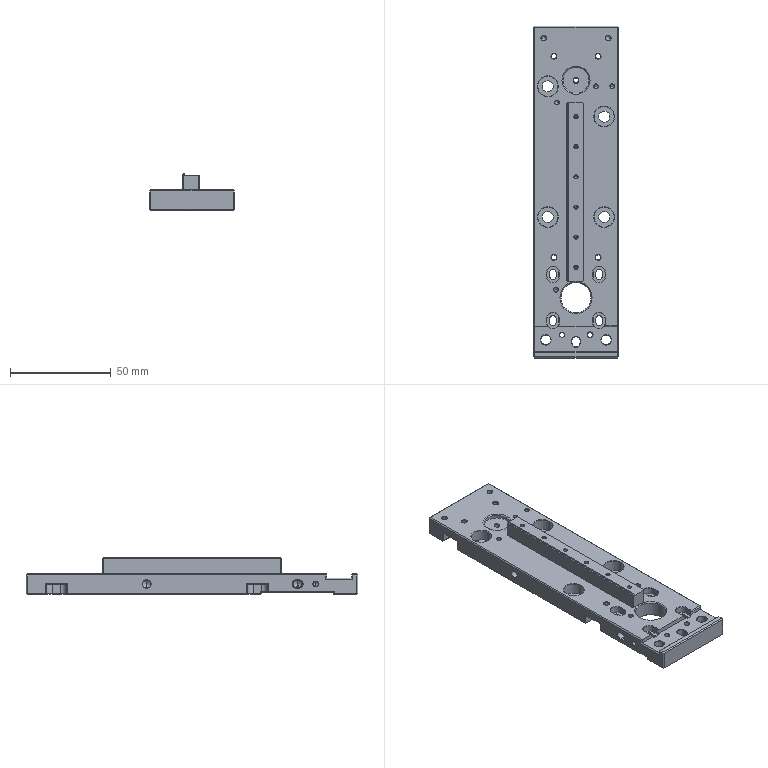Part | SolidWorks | features HoleWzd 13, ICE 13, Chamfer 2, Extrusion 1 | 1 solid | 483 faces | box 42 x 165 x 18 mm | volume 61836 mm3 | plane 209 | cone 162 | cylinder 112 | commonest cylinder face diameters 2.5 x24 6 x16 1.6 x12 4 x11 2.05 x8 3.2 x8